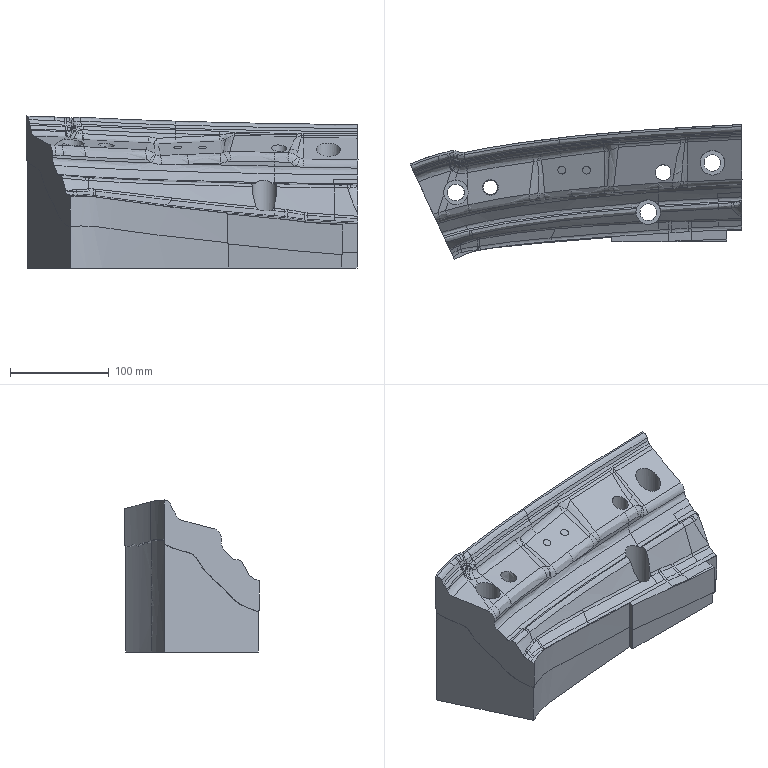Part | NX | features solid 2 | 1 solid | 236 faces | box 336.591 x 136.581 x 154.109 mm | volume 3401336 mm3 | spline 209 | plane 17 | cylinder 10 | commonest cylinder face diameters 25 x6 17 x3 16 x1